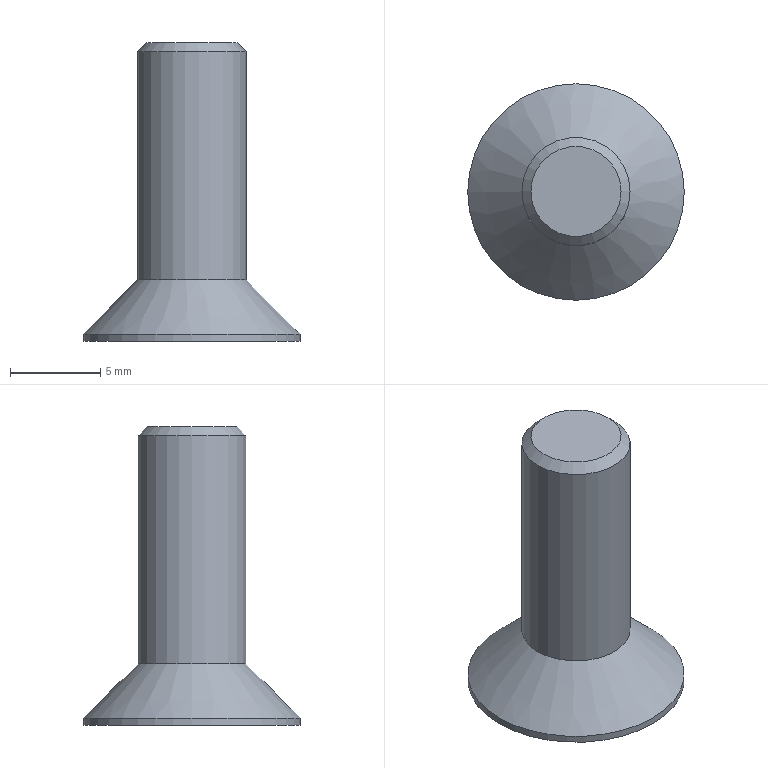Part | STEP file | PTM6.00-15.00 | 1 solid | 13 faces | box 12 x 12 x 16.55 mm | volume 586.414 mm3 | plane 9 | cone 2 | cylinder 2 | commonest cylinder face diameters 6 x1 12 x1